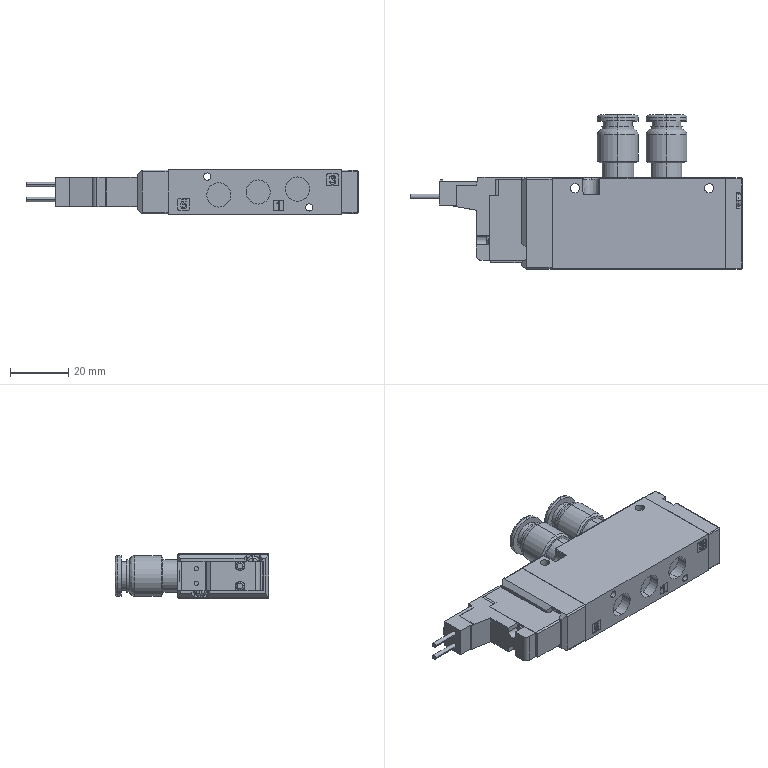Part | STEP file | 4RD219-GS8-E2-3_default | 13 solids | 686 faces | box 113.84 x 52.8 x 15.298 mm | volume 41991 mm3 | plane 320 | cylinder 223 | spline 90 | cone 53 | commonest cylinder face diameters 0.6 x44 2.5 x20 8.3 x10 1 x8 2.208 x8 2.6 x8